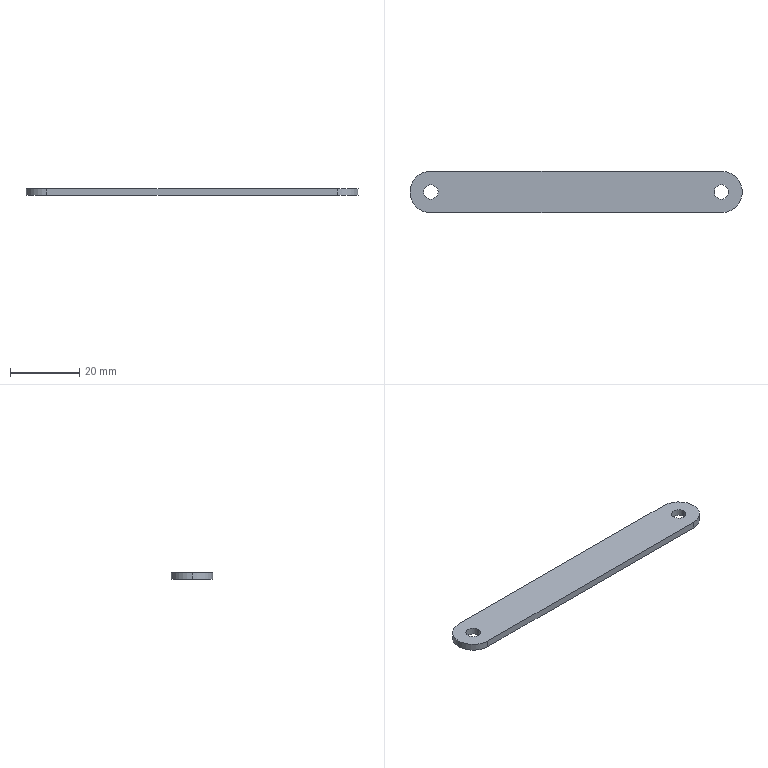Part | SolidWorks | features Extrusion 1, HoleWzd 1 | 1 solid | 11 faces | box 96 x 12 x 2 mm | volume 2187 mm3 | cylinder 7 | plane 4 | commonest cylinder face diameters 4.2 x4 12 x3
STEP:
#1=CARTESIAN_POINT('',(-2.1,0.,-1.));
#2=VERTEX_POINT('',#1);
#3=CARTESIAN_POINT('',(2.1,0.,-1.));
#4=VERTEX_POINT('',#3);
#5=CARTESIAN_POINT('',(0.,0.,-1.));
#6=DIRECTION('',(0.,0.,1.));
#7=DIRECTION('',(1.,0.,0.));
#8=AXIS2_PLACEMENT_3D('',#5,#6,#7);
#9=CIRCLE('',#8,2.1);
#10=EDGE_CURVE('',#2,#4,#9,.T.);
#11=ORIENTED_EDGE('',*,*,#10,.F.);
#12=CARTESIAN_POINT('',(-2.1,0.,1.));
#13=VERTEX_POINT('',#12);
#14=CARTESIAN_POINT('',(-2.1,0.,1.));
#15=DIRECTION('',(0.,0.,1.));
#16=VECTOR('',#15,1000.);
#17=LINE('',#14,#16);
#18=EDGE_CURVE('',#2,#13,#17,.T.);
#19=ORIENTED_EDGE('',*,*,#18,.T.);
#20=CARTESIAN_POINT('',(2.1,0.,1.));
#21=VERTEX_POINT('',#20);
#22=CARTESIAN_POINT('',(0.,0.,1.));
#23=DIRECTION('',(0.,0.,1.));
#24=DIRECTION('',(1.,0.,0.));
#25=AXIS2_PLACEMENT_3D('',#22,#23,#24);
#26=CIRCLE('',#25,2.1);
#27=EDGE_CURVE('',#13,#21,#26,.T.);
#28=ORIENTED_EDGE('',*,*,#27,.T.);
#29=CARTESIAN_POINT('',(2.1,0.,1.));
#30=DIRECTION('',(0.,0.,1.));
#31=VECTOR('',#30,1000.);
#32=LINE('',#29,#31);
#33=EDGE_CURVE('',#4,#21,#32,.T.);
#34=ORIENTED_EDGE('',*,*,#33,.F.);
#35=EDGE_LOOP('',(#11,#19,#28,#34));
#36=FACE_OUTER_BOUND('',#35,.T.);
#37=CARTESIAN_POINT('',(0.,0.,1.));
#38=DIRECTION('',(0.,0.,1.));
#39=DIRECTION('',(1.,0.,0.));
#40=AXIS2_PLACEMENT_3D('',#37,#38,#39);
#41=CYLINDRICAL_SURFACE('',#40,2.1);
#42=ADVANCED_FACE('',(#36),#41,.F.);
#43=CARTESIAN_POINT('',(81.9,0.,-1.));
#44=VERTEX_POINT('',#43);
#45=CARTESIAN_POINT('',(86.1,0.,-1.));
#46=VERTEX_POINT('',#45);
#47=CARTESIAN_POINT('',(84.,0.,-1.));
#48=DIRECTION('',(0.,0.,1.));
#49=DIRECTION('',(1.,0.,0.));
#50=AXIS2_PLACEMENT_3D('',#47,#48,#49);
#51=CIRCLE('',#50,2.1);
#52=EDGE_CURVE('',#44,#46,#51,.T.);
#53=ORIENTED_EDGE('',*,*,#52,.F.);
#54=CARTESIAN_POINT('',(81.9,0.,1.));
#55=VERTEX_POINT('',#54);
#56=CARTESIAN_POINT('',(81.9,0.,1.));
#57=DIRECTION('',(0.,0.,1.));
#58=VECTOR('',#57,1000.);
#59=LINE('',#56,#58);
#60=EDGE_CURVE('',#44,#55,#59,.T.);
#61=ORIENTED_EDGE('',*,*,#60,.T.);
#62=CARTESIAN_POINT('',(86.1,0.,1.));
#63=VERTEX_POINT('',#62);
#64=CARTESIAN_POINT('',(84.,0.,1.));
#65=DIRECTION('',(0.,0.,1.));
#66=DIRECTION('',(1.,0.,0.));
#67=AXIS2_PLACEMENT_3D('',#64,#65,#66);
#68=CIRCLE('',#67,2.1);
#69=EDGE_CURVE('',#55,#63,#68,.T.);
#70=ORIENTED_EDGE('',*,*,#69,.T.);
#71=CARTESIAN_POINT('',(86.1,0.,1.));
#72=DIRECTION('',(0.,0.,1.));
#73=VECTOR('',#72,1000.);
#74=LINE('',#71,#73);
#75=EDGE_CURVE('',#46,#63,#74,.T.);
#76=ORIENTED_EDGE('',*,*,#75,.F.);
#77=EDGE_LOOP('',(#53,#61,#70,#76));
#78=FACE_OUTER_BOUND('',#77,.T.);
#79=CARTESIAN_POINT('',(84.,0.,1.));
#80=DIRECTION('',(0.,0.,1.));
#81=DIRECTION('',(1.,0.,0.));
#82=AXIS2_PLACEMENT_3D('',#79,#80,#81);
#83=CYLINDRICAL_SURFACE('',#82,2.1);
#84=ADVANCED_FACE('',(#78),#83,.F.);
#85=CARTESIAN_POINT('',(-6.,0.,1.));
#86=VERTEX_POINT('',#85);
#87=CARTESIAN_POINT('',(0.,-6.,1.));
#88=VERTEX_POINT('',#87);
#89=CARTESIAN_POINT('',(0.,0.,1.));
#90=DIRECTION('',(0.,0.,1.));
#91=DIRECTION('',(1.,0.,0.));
#92=AXIS2_PLACEMENT_3D('',#89,#90,#91);
#93=CIRCLE('',#92,6.);
#94=EDGE_CURVE('',#86,#88,#93,.T.);
#95=ORIENTED_EDGE('',*,*,#94,.F.);
#96=CARTESIAN_POINT('',(-6.,0.,-1.));
#97=VERTEX_POINT('',#96);
#98=CARTESIAN_POINT('',(-6.,0.,1.));
#99=DIRECTION('',(0.,0.,-1.));
#100=VECTOR('',#99,1000.);
#101=LINE('',#98,#100);
#102=EDGE_CURVE('',#86,#97,#101,.T.);
#103=ORIENTED_EDGE('',*,*,#102,.T.);
#104=CARTESIAN_POINT('',(0.,-6.,-1.));
#105=VERTEX_POINT('',#104);
#106=CARTESIAN_POINT('',(0.,0.,-1.));
#107=DIRECTION('',(0.,0.,1.));
#108=DIRECTION('',(1.,0.,0.));
#109=AXIS2_PLACEMENT_3D('',#106,#107,#108);
#110=CIRCLE('',#109,6.);
#111=EDGE_CURVE('',#97,#105,#110,.T.);
#112=ORIENTED_EDGE('',*,*,#111,.T.);
#113=CARTESIAN_POINT('',(0.,-6.,1.));
#114=DIRECTION('',(0.,0.,-1.));
#115=VECTOR('',#114,1000.);
#116=LINE('',#113,#115);
#117=EDGE_CURVE('',#88,#105,#116,.T.);
#118=ORIENTED_EDGE('',*,*,#117,.F.);
#119=EDGE_LOOP('',(#95,#103,#112,#118));
#120=FACE_OUTER_BOUND('',#119,.T.);
#121=CARTESIAN_POINT('',(0.,0.,1.));
#122=DIRECTION('',(0.,0.,-1.));
#123=DIRECTION('',(-1.,0.,0.));
#124=AXIS2_PLACEMENT_3D('',#121,#122,#123);
#125=CYLINDRICAL_SURFACE('',#124,6.);
#126=ADVANCED_FACE('',(#120),#125,.T.);
#127=ORIENTED_EDGE('',*,*,#102,.F.);
#128=CARTESIAN_POINT('',(0.,6.,1.));
#129=VERTEX_POINT('',#128);
#130=CARTESIAN_POINT('',(0.,0.,1.));
#131=DIRECTION('',(0.,0.,1.));
#132=DIRECTION('',(1.,0.,0.));
#133=AXIS2_PLACEMENT_3D('',#130,#131,#132);
#134=CIRCLE('',#133,6.);
#135=EDGE_CURVE('',#129,#86,#134,.T.);
#136=ORIENTED_EDGE('',*,*,#135,.F.);
#137=CARTESIAN_POINT('',(0.,6.,-1.));
#138=VERTEX_POINT('',#137);
#139=CARTESIAN_POINT('',(0.,6.,1.));
#140=DIRECTION('',(0.,0.,-1.));
#141=VECTOR('',#140,1000.);
#142=LINE('',#139,#141);
#143=EDGE_CURVE('',#129,#138,#142,.T.);
#144=ORIENTED_EDGE('',*,*,#143,.T.);
#145=CARTESIAN_POINT('',(0.,0.,-1.));
#146=DIRECTION('',(0.,0.,1.));
#147=DIRECTION('',(1.,0.,0.));
#148=AXIS2_PLACEMENT_3D('',#145,#146,#147);
#149=CIRCLE('',#148,6.);
#150=EDGE_CURVE('',#138,#97,#149,.T.);
#151=ORIENTED_EDGE('',*,*,#150,.T.);
#152=EDGE_LOOP('',(#127,#136,#144,#151));
#153=FACE_OUTER_BOUND('',#152,.T.);
#154=CARTESIAN_POINT('',(0.,0.,1.));
#155=DIRECTION('',(0.,0.,-1.));
#156=DIRECTION('',(-1.,0.,0.));
#157=AXIS2_PLACEMENT_3D('',#154,#155,#156);
#158=CYLINDRICAL_SURFACE('',#157,6.);
#159=ADVANCED_FACE('',(#153),#158,.T.);
#160=CARTESIAN_POINT('',(84.,-6.,-1.));
#161=VERTEX_POINT('',#160);
#162=CARTESIAN_POINT('',(0.,-6.,-1.));
#163=DIRECTION('',(1.,0.,0.));
#164=VECTOR('',#163,1000.);
#165=LINE('',#162,#164);
#166=EDGE_CURVE('',#105,#161,#165,.T.);
#167=ORIENTED_EDGE('',*,*,#166,.T.);
#168=CARTESIAN_POINT('',(84.,-6.,1.));
#169=VERTEX_POINT('',#168);
#170=CARTESIAN_POINT('',(84.,-6.,1.));
#171=DIRECTION('',(0.,0.,-1.));
#172=VECTOR('',#171,1000.);
#173=LINE('',#170,#172);
#174=EDGE_CURVE('',#169,#161,#173,.T.);
#175=ORIENTED_EDGE('',*,*,#174,.F.);
#176=CARTESIAN_POINT('',(0.,-6.,1.));
#177=DIRECTION('',(1.,0.,0.));
#178=VECTOR('',#177,1000.);
#179=LINE('',#176,#178);
#180=EDGE_CURVE('',#88,#169,#179,.T.);
#181=ORIENTED_EDGE('',*,*,#180,.F.);
#182=ORIENTED_EDGE('',*,*,#117,.T.);
#183=EDGE_LOOP('',(#167,#175,#181,#182));
#184=FACE_OUTER_BOUND('',#183,.T.);
#185=CARTESIAN_POINT('',(0.,-6.,1.));
#186=DIRECTION('',(0.,1.,0.));
#187=DIRECTION('',(0.,0.,1.));
#188=AXIS2_PLACEMENT_3D('',#185,#186,#187);
#189=PLANE('',#188);
#190=ADVANCED_FACE('',(#184),#189,.F.);
#191=CARTESIAN_POINT('',(84.,6.,-1.));
#192=VERTEX_POINT('',#191);
#193=CARTESIAN_POINT('',(84.,0.,-1.));
#194=DIRECTION('',(0.,0.,1.));
#195=DIRECTION('',(1.,0.,0.));
#196=AXIS2_PLACEMENT_3D('',#193,#194,#195);
#197=CIRCLE('',#196,6.);
#198=EDGE_CURVE('',#161,#192,#197,.T.);
#199=ORIENTED_EDGE('',*,*,#198,.T.);
#200=CARTESIAN_POINT('',(84.,6.,1.));
#201=VERTEX_POINT('',#200);
#202=CARTESIAN_POINT('',(84.,6.,1.));
#203=DIRECTION('',(0.,0.,-1.));
#204=VECTOR('',#203,1000.);
#205=LINE('',#202,#204);
#206=EDGE_CURVE('',#201,#192,#205,.T.);
#207=ORIENTED_EDGE('',*,*,#206,.F.);
#208=CARTESIAN_POINT('',(84.,0.,1.));
#209=DIRECTION('',(0.,0.,1.));
#210=DIRECTION('',(1.,0.,0.));
#211=AXIS2_PLACEMENT_3D('',#208,#209,#210);
#212=CIRCLE('',#211,6.);
#213=EDGE_CURVE('',#169,#201,#212,.T.);
#214=ORIENTED_EDGE('',*,*,#213,.F.);
#215=ORIENTED_EDGE('',*,*,#174,.T.);
#216=EDGE_LOOP('',(#199,#207,#214,#215));
#217=FACE_OUTER_BOUND('',#216,.T.);
#218=CARTESIAN_POINT('',(84.,0.,1.));
#219=DIRECTION('',(0.,0.,-1.));
#220=DIRECTION('',(-1.,0.,0.));
#221=AXIS2_PLACEMENT_3D('',#218,#219,#220);
#222=CYLINDRICAL_SURFACE('',#221,6.);
#223=ADVANCED_FACE('',(#217),#222,.T.);
#224=CARTESIAN_POINT('',(0.,6.,-1.));
#225=DIRECTION('',(-1.,0.,0.));
#226=VECTOR('',#225,1000.);
#227=LINE('',#224,#226);
#228=EDGE_CURVE('',#192,#138,#227,.T.);
#229=ORIENTED_EDGE('',*,*,#228,.T.);
#230=ORIENTED_EDGE('',*,*,#143,.F.);
#231=CARTESIAN_POINT('',(0.,6.,1.));
#232=DIRECTION('',(-1.,0.,0.));
#233=VECTOR('',#232,1000.);
#234=LINE('',#231,#233);
#235=EDGE_CURVE('',#201,#129,#234,.T.);
#236=ORIENTED_EDGE('',*,*,#235,.F.);
#237=ORIENTED_EDGE('',*,*,#206,.T.);
#238=EDGE_LOOP('',(#229,#230,#236,#237));
#239=FACE_OUTER_BOUND('',#238,.T.);
#240=CARTESIAN_POINT('',(0.,6.,1.));
#241=DIRECTION('',(0.,-1.,0.));
#242=DIRECTION('',(0.,0.,-1.));
#243=AXIS2_PLACEMENT_3D('',#240,#241,#242);
#244=PLANE('',#243);
#245=ADVANCED_FACE('',(#239),#244,.F.);
#246=CARTESIAN_POINT('',(0.,0.,1.));
#247=DIRECTION('',(0.,0.,1.));
#248=DIRECTION('',(1.,0.,0.));
#249=AXIS2_PLACEMENT_3D('',#246,#247,#248);
#250=CIRCLE('',#249,2.1);
#251=EDGE_CURVE('',#21,#13,#250,.T.);
#252=ORIENTED_EDGE('',*,*,#251,.F.);
#253=ORIENTED_EDGE('',*,*,#27,.F.);
#254=EDGE_LOOP('',(#252,#253));
#255=FACE_BOUND('',#254,.T.);
#256=CARTESIAN_POINT('',(84.,0.,1.));
#257=DIRECTION('',(0.,0.,1.));
#258=DIRECTION('',(1.,0.,0.));
#259=AXIS2_PLACEMENT_3D('',#256,#257,#258);
#260=CIRCLE('',#259,2.1);
#261=EDGE_CURVE('',#63,#55,#260,.T.);
#262=ORIENTED_EDGE('',*,*,#261,.F.);
#263=ORIENTED_EDGE('',*,*,#69,.F.);
#264=EDGE_LOOP('',(#262,#263));
#265=FACE_BOUND('',#264,.T.);
#266=ORIENTED_EDGE('',*,*,#135,.T.);
#267=ORIENTED_EDGE('',*,*,#94,.T.);
#268=ORIENTED_EDGE('',*,*,#180,.T.);
#269=ORIENTED_EDGE('',*,*,#213,.T.);
#270=ORIENTED_EDGE('',*,*,#235,.T.);
#271=EDGE_LOOP('',(#266,#267,#268,#269,#270));
#272=FACE_OUTER_BOUND('',#271,.T.);
#273=CARTESIAN_POINT('',(0.,0.,1.));
#274=DIRECTION('',(0.,0.,1.));
#275=DIRECTION('',(1.,0.,0.));
#276=AXIS2_PLACEMENT_3D('',#273,#274,#275);
#277=PLANE('',#276);
#278=ADVANCED_FACE('',(#255,#265,#272),#277,.T.);
#279=CARTESIAN_POINT('',(0.,0.,-1.));
#280=DIRECTION('',(0.,0.,1.));
#281=DIRECTION('',(1.,0.,0.));
#282=AXIS2_PLACEMENT_3D('',#279,#280,#281);
#283=CIRCLE('',#282,2.1);
#284=EDGE_CURVE('',#4,#2,#283,.T.);
#285=ORIENTED_EDGE('',*,*,#284,.T.);
#286=ORIENTED_EDGE('',*,*,#10,.T.);
#287=EDGE_LOOP('',(#285,#286));
#288=FACE_BOUND('',#287,.T.);
#289=CARTESIAN_POINT('',(84.,0.,-1.));
#290=DIRECTION('',(0.,0.,1.));
#291=DIRECTION('',(1.,0.,0.));
#292=AXIS2_PLACEMENT_3D('',#289,#290,#291);
#293=CIRCLE('',#292,2.1);
#294=EDGE_CURVE('',#46,#44,#293,.T.);
#295=ORIENTED_EDGE('',*,*,#294,.T.);
#296=ORIENTED_EDGE('',*,*,#52,.T.);
#297=EDGE_LOOP('',(#295,#296));
#298=FACE_BOUND('',#297,.T.);
#299=ORIENTED_EDGE('',*,*,#150,.F.);
#300=ORIENTED_EDGE('',*,*,#228,.F.);
#301=ORIENTED_EDGE('',*,*,#198,.F.);
#302=ORIENTED_EDGE('',*,*,#166,.F.);
#303=ORIENTED_EDGE('',*,*,#111,.F.);
#304=EDGE_LOOP('',(#299,#300,#301,#302,#303));
#305=FACE_OUTER_BOUND('',#304,.T.);
#306=CARTESIAN_POINT('',(0.,0.,-1.));
#307=DIRECTION('',(0.,0.,1.));
#308=DIRECTION('',(1.,0.,0.));
#309=AXIS2_PLACEMENT_3D('',#306,#307,#308);
#310=PLANE('',#309);
#311=ADVANCED_FACE('',(#288,#298,#305),#310,.F.);
#312=ORIENTED_EDGE('',*,*,#60,.F.);
#313=ORIENTED_EDGE('',*,*,#294,.F.);
#314=ORIENTED_EDGE('',*,*,#75,.T.);
#315=ORIENTED_EDGE('',*,*,#261,.T.);
#316=EDGE_LOOP('',(#312,#313,#314,#315));
#317=FACE_OUTER_BOUND('',#316,.T.);
#318=CARTESIAN_POINT('',(84.,0.,1.));
#319=DIRECTION('',(0.,0.,1.));
#320=DIRECTION('',(1.,0.,0.));
#321=AXIS2_PLACEMENT_3D('',#318,#319,#320);
#322=CYLINDRICAL_SURFACE('',#321,2.1);
#323=ADVANCED_FACE('',(#317),#322,.F.);
#324=ORIENTED_EDGE('',*,*,#18,.F.);
#325=ORIENTED_EDGE('',*,*,#284,.F.);
#326=ORIENTED_EDGE('',*,*,#33,.T.);
#327=ORIENTED_EDGE('',*,*,#251,.T.);
#328=EDGE_LOOP('',(#324,#325,#326,#327));
#329=FACE_OUTER_BOUND('',#328,.T.);
#330=CARTESIAN_POINT('',(0.,0.,1.));
#331=DIRECTION('',(0.,0.,1.));
#332=DIRECTION('',(1.,0.,0.));
#333=AXIS2_PLACEMENT_3D('',#330,#331,#332);
#334=CYLINDRICAL_SURFACE('',#333,2.1);
#335=ADVANCED_FACE('',(#329),#334,.F.);
#336=CLOSED_SHELL('',(#42,#84,#126,#159,#190,#223,#245,#278,#311,#323,#335));
#337=MANIFOLD_SOLID_BREP('',#336);
#338=CARTESIAN_POINT('',(0.,0.,0.));
#339=DIRECTION('',(0.,0.,1.));
#340=DIRECTION('',(1.,0.,0.));
#341=AXIS2_PLACEMENT_3D('',#338,#339,#340);
#342=(LENGTH_UNIT()NAMED_UNIT(*)SI_UNIT(.MILLI.,.METRE.));
#343=UNCERTAINTY_MEASURE_WITH_UNIT(LENGTH_MEASURE(0.00001),#342,'','');
#344=(NAMED_UNIT(*)PLANE_ANGLE_UNIT()SI_UNIT($,.RADIAN.));
#345=(NAMED_UNIT(*)SI_UNIT($,.STERADIAN.)SOLID_ANGLE_UNIT());
#346=(GEOMETRIC_REPRESENTATION_CONTEXT(3)GLOBAL_UNCERTAINTY_ASSIGNED_CONTEXT((#343))GLOBAL_UNIT_ASSIGNED_CONTEXT((#342,#344,#345))REPRESENTATION_CONTEXT('',''));
#347=ADVANCED_BREP_SHAPE_REPRESENTATION('',(#337,#341),#346);